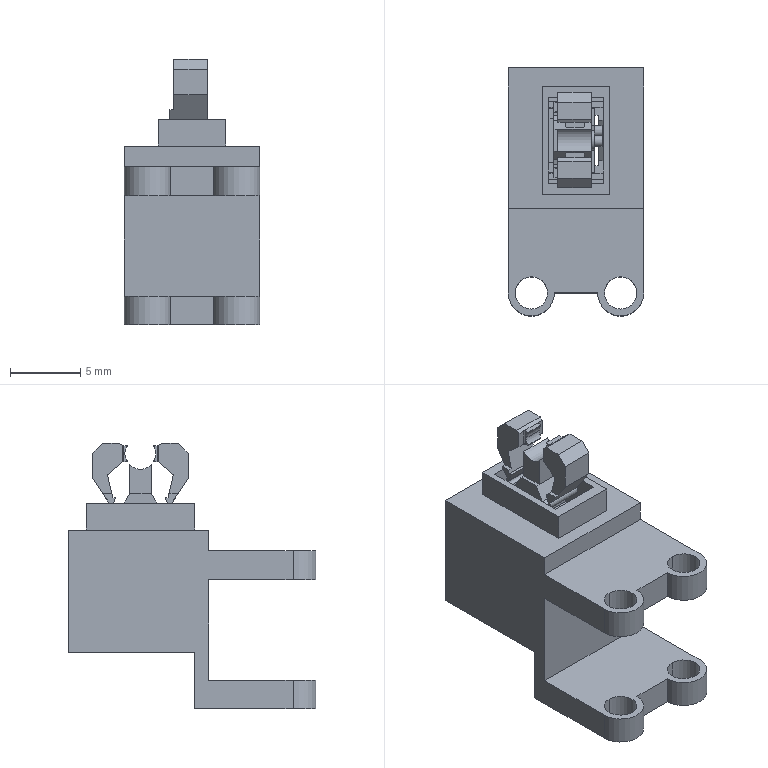Part | SolidWorks | 5 solids | 239 faces | box 9.63 x 17.64 x 18.86 mm | volume 1059 mm3 | plane 189 | cylinder 46 | cone 2 | spline 2 | commonest cylinder face diameters 2.3 x8 0.91 x6 1.4 x5 0.14 x4 3.28 x4 0.42 x3